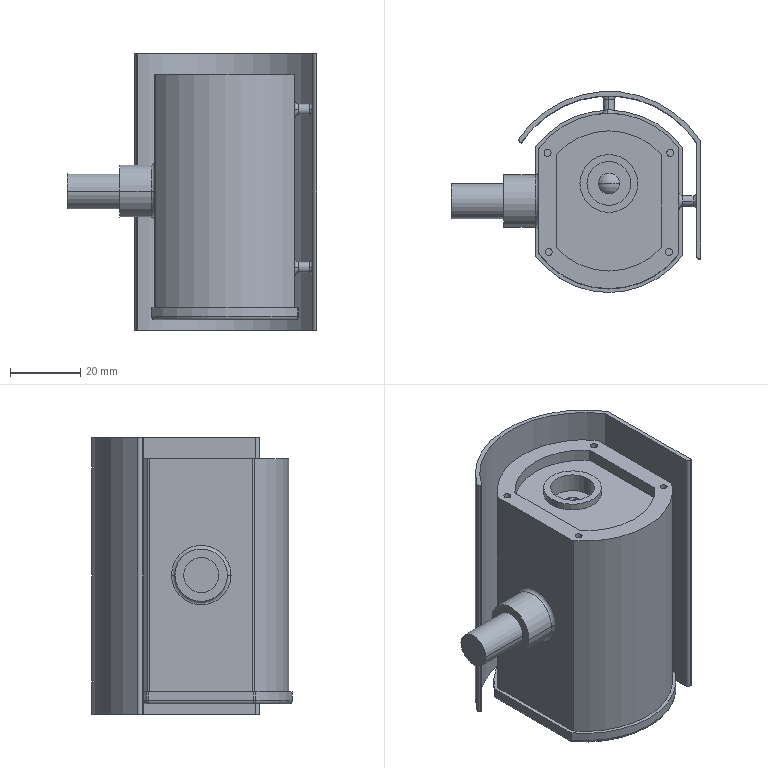Part | SolidWorks | features ICE 14, Dome 1, Extrusion 1, Fillet 1, Scale 1 | 1 solid | 190 faces | box 71.25 x 57.25 x 79 mm | volume 129826 mm3 | plane 94 | cylinder 70 | torus 12 | spline 8 | sphere 6 | commonest cylinder face diameters 2 x29 3 x12 45 x11 6 x2 10 x2 12.5 x2